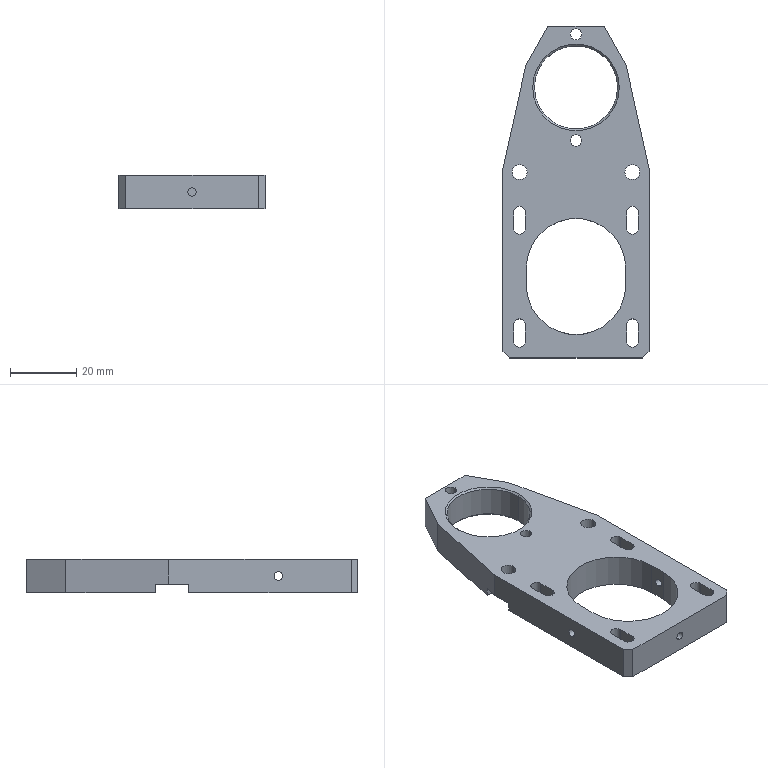Part | SolidWorks | features ICE 7, HoleWzd 5, Chamfer 2, MirrorPattern 2, Cut 1, Extrusion 1, LPattern 1 | 1 solid | 83 faces | box 44 x 100 x 10 mm | volume 22505 mm3 | plane 42 | cylinder 37 | cone 4 | commonest cylinder face diameters 3.5 x8 5.8 x8 2.5 x6 3.4 x4 4.5 x4 6 x3